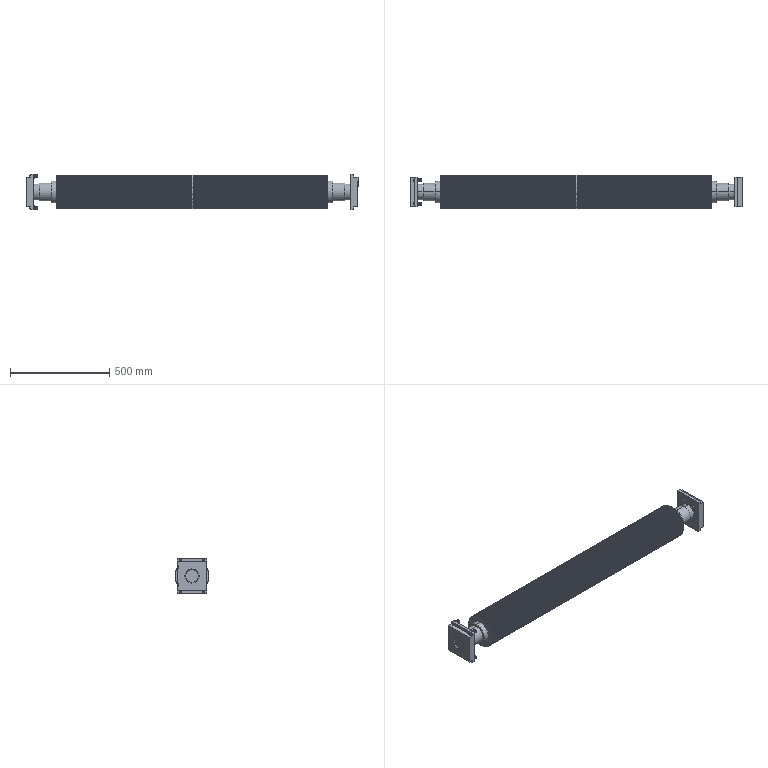Part | SolidWorks | 50 solids | 1337 faces | box 1672 x 169.976 x 180 mm | volume 33756798 mm3 | cylinder 791 | plane 190 | cone 152 | sphere 144 | torus 60 | commonest cylinder face diameters 1 x288 2 x167 170 x120 89.75 x66 95.25 x66 10 x16